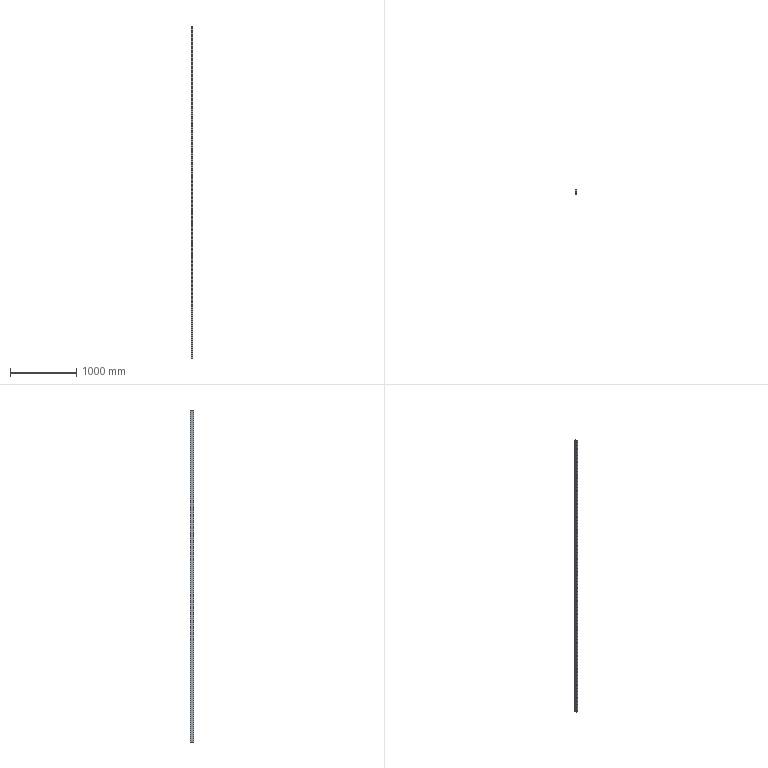Part | SolidWorks | features BaseBody 1 | 1 solid | 342 faces | box 30 x 55 x 5030 mm | volume 8266814 mm3 | cone 168 | cylinder 168 | plane 6 | commonest cylinder face diameters 4.917 x168